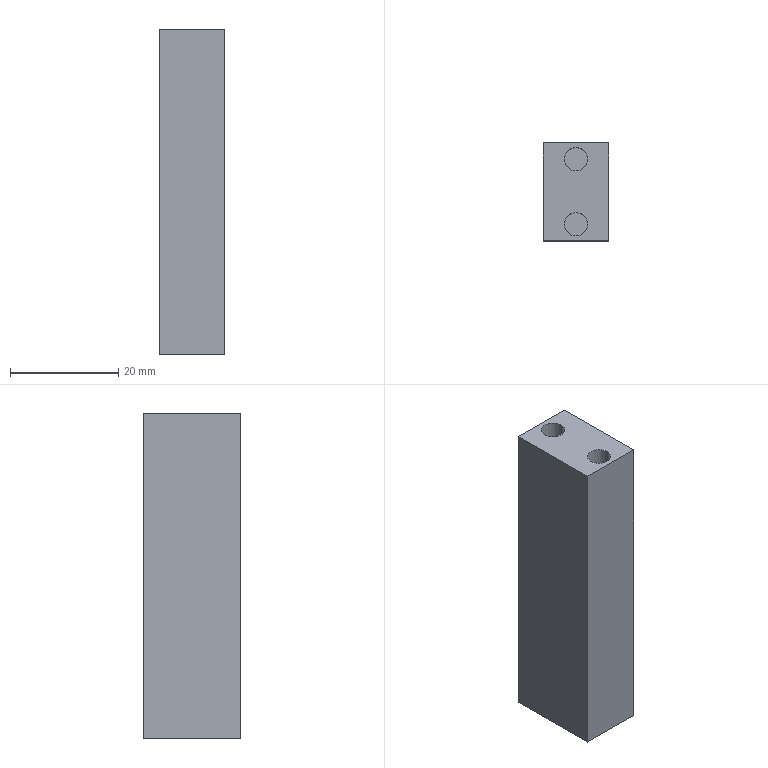Part | SolidWorks | features BaseBody 1 | 1 solid | 12 faces | box 12 x 18 x 60 mm | volume 12664 mm3 | plane 8 | cylinder 4 | commonest cylinder face diameters 4.3 x4
STEP:
#1=CARTESIAN_POINT('',(-2.15,6.,19.8));
#2=VERTEX_POINT('',#1);
#3=CARTESIAN_POINT('',(2.15,6.,19.8));
#4=VERTEX_POINT('',#3);
#5=CARTESIAN_POINT('',(0.,6.,19.8));
#6=DIRECTION('',(0.,0.,1.));
#7=DIRECTION('',(1.,0.,0.));
#8=AXIS2_PLACEMENT_3D('',#5,#6,#7);
#9=CIRCLE('',#8,2.15);
#10=EDGE_CURVE('',#2,#4,#9,.T.);
#11=ORIENTED_EDGE('',*,*,#10,.F.);
#12=CARTESIAN_POINT('',(-2.15,6.,30.));
#13=VERTEX_POINT('',#12);
#14=CARTESIAN_POINT('',(-2.15,6.,19.8));
#15=DIRECTION('',(0.,0.,1.));
#16=VECTOR('',#15,1000.);
#17=LINE('',#14,#16);
#18=EDGE_CURVE('',#2,#13,#17,.T.);
#19=ORIENTED_EDGE('',*,*,#18,.T.);
#20=CARTESIAN_POINT('',(2.15,6.,30.));
#21=VERTEX_POINT('',#20);
#22=CARTESIAN_POINT('',(0.,6.,30.));
#23=DIRECTION('',(0.,0.,-1.));
#24=DIRECTION('',(1.,0.,0.));
#25=AXIS2_PLACEMENT_3D('',#22,#23,#24);
#26=CIRCLE('',#25,2.15);
#27=EDGE_CURVE('',#21,#13,#26,.T.);
#28=ORIENTED_EDGE('',*,*,#27,.F.);
#29=CARTESIAN_POINT('',(2.15,6.,19.8));
#30=DIRECTION('',(0.,0.,1.));
#31=VECTOR('',#30,1000.);
#32=LINE('',#29,#31);
#33=EDGE_CURVE('',#4,#21,#32,.T.);
#34=ORIENTED_EDGE('',*,*,#33,.F.);
#35=EDGE_LOOP('',(#11,#19,#28,#34));
#36=FACE_OUTER_BOUND('',#35,.T.);
#37=CARTESIAN_POINT('',(0.,6.,19.8));
#38=DIRECTION('',(0.,0.,1.));
#39=DIRECTION('',(1.,0.,0.));
#40=AXIS2_PLACEMENT_3D('',#37,#38,#39);
#41=CYLINDRICAL_SURFACE('',#40,2.15);
#42=ADVANCED_FACE('',(#36),#41,.F.);
#43=CARTESIAN_POINT('',(-2.15,-6.,19.8));
#44=VERTEX_POINT('',#43);
#45=CARTESIAN_POINT('',(2.15,-6.,19.8));
#46=VERTEX_POINT('',#45);
#47=CARTESIAN_POINT('',(0.,-6.,19.8));
#48=DIRECTION('',(0.,0.,1.));
#49=DIRECTION('',(1.,0.,0.));
#50=AXIS2_PLACEMENT_3D('',#47,#48,#49);
#51=CIRCLE('',#50,2.15);
#52=EDGE_CURVE('',#44,#46,#51,.T.);
#53=ORIENTED_EDGE('',*,*,#52,.F.);
#54=CARTESIAN_POINT('',(-2.15,-6.,30.));
#55=VERTEX_POINT('',#54);
#56=CARTESIAN_POINT('',(-2.15,-6.,19.8));
#57=DIRECTION('',(0.,0.,1.));
#58=VECTOR('',#57,1000.);
#59=LINE('',#56,#58);
#60=EDGE_CURVE('',#44,#55,#59,.T.);
#61=ORIENTED_EDGE('',*,*,#60,.T.);
#62=CARTESIAN_POINT('',(2.15,-6.,30.));
#63=VERTEX_POINT('',#62);
#64=CARTESIAN_POINT('',(0.,-6.,30.));
#65=DIRECTION('',(0.,0.,-1.));
#66=DIRECTION('',(1.,0.,0.));
#67=AXIS2_PLACEMENT_3D('',#64,#65,#66);
#68=CIRCLE('',#67,2.15);
#69=EDGE_CURVE('',#63,#55,#68,.T.);
#70=ORIENTED_EDGE('',*,*,#69,.F.);
#71=CARTESIAN_POINT('',(2.15,-6.,19.8));
#72=DIRECTION('',(0.,0.,1.));
#73=VECTOR('',#72,1000.);
#74=LINE('',#71,#73);
#75=EDGE_CURVE('',#46,#63,#74,.T.);
#76=ORIENTED_EDGE('',*,*,#75,.F.);
#77=EDGE_LOOP('',(#53,#61,#70,#76));
#78=FACE_OUTER_BOUND('',#77,.T.);
#79=CARTESIAN_POINT('',(0.,-6.,19.8));
#80=DIRECTION('',(0.,0.,1.));
#81=DIRECTION('',(1.,0.,0.));
#82=AXIS2_PLACEMENT_3D('',#79,#80,#81);
#83=CYLINDRICAL_SURFACE('',#82,2.15);
#84=ADVANCED_FACE('',(#78),#83,.F.);
#85=CARTESIAN_POINT('',(-6.,9.,-30.));
#86=VERTEX_POINT('',#85);
#87=CARTESIAN_POINT('',(-6.,9.,30.));
#88=VERTEX_POINT('',#87);
#89=CARTESIAN_POINT('',(-6.,9.,-30.));
#90=DIRECTION('',(0.,0.,1.));
#91=VECTOR('',#90,1000.);
#92=LINE('',#89,#91);
#93=EDGE_CURVE('',#86,#88,#92,.T.);
#94=ORIENTED_EDGE('',*,*,#93,.F.);
#95=CARTESIAN_POINT('',(-6.,-9.,-30.));
#96=VERTEX_POINT('',#95);
#97=CARTESIAN_POINT('',(-6.,-9.,-30.));
#98=DIRECTION('',(0.,1.,0.));
#99=VECTOR('',#98,1000.);
#100=LINE('',#97,#99);
#101=EDGE_CURVE('',#96,#86,#100,.T.);
#102=ORIENTED_EDGE('',*,*,#101,.F.);
#103=CARTESIAN_POINT('',(-6.,-9.,30.));
#104=VERTEX_POINT('',#103);
#105=CARTESIAN_POINT('',(-6.,-9.,-30.));
#106=DIRECTION('',(0.,0.,-1.));
#107=VECTOR('',#106,1000.);
#108=LINE('',#105,#107);
#109=EDGE_CURVE('',#104,#96,#108,.T.);
#110=ORIENTED_EDGE('',*,*,#109,.F.);
#111=CARTESIAN_POINT('',(-6.,-9.,30.));
#112=DIRECTION('',(0.,-1.,0.));
#113=VECTOR('',#112,1000.);
#114=LINE('',#111,#113);
#115=EDGE_CURVE('',#88,#104,#114,.T.);
#116=ORIENTED_EDGE('',*,*,#115,.F.);
#117=EDGE_LOOP('',(#94,#102,#110,#116));
#118=FACE_OUTER_BOUND('',#117,.T.);
#119=CARTESIAN_POINT('',(-6.,-9.,-30.));
#120=DIRECTION('',(1.,0.,0.));
#121=DIRECTION('',(0.,0.,-1.));
#122=AXIS2_PLACEMENT_3D('',#119,#120,#121);
#123=PLANE('',#122);
#124=ADVANCED_FACE('',(#118),#123,.F.);
#125=ORIENTED_EDGE('',*,*,#27,.T.);
#126=CARTESIAN_POINT('',(0.,6.,30.));
#127=DIRECTION('',(0.,0.,-1.));
#128=DIRECTION('',(1.,0.,0.));
#129=AXIS2_PLACEMENT_3D('',#126,#127,#128);
#130=CIRCLE('',#129,2.15);
#131=EDGE_CURVE('',#13,#21,#130,.T.);
#132=ORIENTED_EDGE('',*,*,#131,.T.);
#133=EDGE_LOOP('',(#125,#132));
#134=FACE_BOUND('',#133,.T.);
#135=ORIENTED_EDGE('',*,*,#69,.T.);
#136=CARTESIAN_POINT('',(0.,-6.,30.));
#137=DIRECTION('',(0.,0.,-1.));
#138=DIRECTION('',(1.,0.,0.));
#139=AXIS2_PLACEMENT_3D('',#136,#137,#138);
#140=CIRCLE('',#139,2.15);
#141=EDGE_CURVE('',#55,#63,#140,.T.);
#142=ORIENTED_EDGE('',*,*,#141,.T.);
#143=EDGE_LOOP('',(#135,#142));
#144=FACE_BOUND('',#143,.T.);
#145=CARTESIAN_POINT('',(6.,-9.,30.));
#146=VERTEX_POINT('',#145);
#147=CARTESIAN_POINT('',(6.,9.,30.));
#148=VERTEX_POINT('',#147);
#149=CARTESIAN_POINT('',(6.,-9.,30.));
#150=DIRECTION('',(0.,1.,0.));
#151=VECTOR('',#150,1000.);
#152=LINE('',#149,#151);
#153=EDGE_CURVE('',#146,#148,#152,.T.);
#154=ORIENTED_EDGE('',*,*,#153,.T.);
#155=CARTESIAN_POINT('',(-6.,9.,30.));
#156=DIRECTION('',(-1.,0.,0.));
#157=VECTOR('',#156,1000.);
#158=LINE('',#155,#157);
#159=EDGE_CURVE('',#148,#88,#158,.T.);
#160=ORIENTED_EDGE('',*,*,#159,.T.);
#161=ORIENTED_EDGE('',*,*,#115,.T.);
#162=CARTESIAN_POINT('',(-6.,-9.,30.));
#163=DIRECTION('',(1.,0.,0.));
#164=VECTOR('',#163,1000.);
#165=LINE('',#162,#164);
#166=EDGE_CURVE('',#104,#146,#165,.T.);
#167=ORIENTED_EDGE('',*,*,#166,.T.);
#168=EDGE_LOOP('',(#154,#160,#161,#167));
#169=FACE_OUTER_BOUND('',#168,.T.);
#170=CARTESIAN_POINT('',(-6.,-9.,30.));
#171=DIRECTION('',(0.,0.,1.));
#172=DIRECTION('',(1.,0.,0.));
#173=AXIS2_PLACEMENT_3D('',#170,#171,#172);
#174=PLANE('',#173);
#175=ADVANCED_FACE('',(#134,#144,#169),#174,.T.);
#176=ORIENTED_EDGE('',*,*,#159,.F.);
#177=CARTESIAN_POINT('',(6.,9.,-30.));
#178=VERTEX_POINT('',#177);
#179=CARTESIAN_POINT('',(6.,9.,-30.));
#180=DIRECTION('',(0.,0.,-1.));
#181=VECTOR('',#180,1000.);
#182=LINE('',#179,#181);
#183=EDGE_CURVE('',#148,#178,#182,.T.);
#184=ORIENTED_EDGE('',*,*,#183,.T.);
#185=CARTESIAN_POINT('',(-6.,9.,-30.));
#186=DIRECTION('',(-1.,0.,0.));
#187=VECTOR('',#186,1000.);
#188=LINE('',#185,#187);
#189=EDGE_CURVE('',#178,#86,#188,.T.);
#190=ORIENTED_EDGE('',*,*,#189,.T.);
#191=ORIENTED_EDGE('',*,*,#93,.T.);
#192=EDGE_LOOP('',(#176,#184,#190,#191));
#193=FACE_OUTER_BOUND('',#192,.T.);
#194=CARTESIAN_POINT('',(-6.,9.,-30.));
#195=DIRECTION('',(0.,1.,0.));
#196=DIRECTION('',(0.,0.,1.));
#197=AXIS2_PLACEMENT_3D('',#194,#195,#196);
#198=PLANE('',#197);
#199=ADVANCED_FACE('',(#193),#198,.T.);
#200=CARTESIAN_POINT('',(6.,-9.,-30.));
#201=VERTEX_POINT('',#200);
#202=CARTESIAN_POINT('',(6.,-9.,-30.));
#203=DIRECTION('',(0.,1.,0.));
#204=VECTOR('',#203,1000.);
#205=LINE('',#202,#204);
#206=EDGE_CURVE('',#201,#178,#205,.T.);
#207=ORIENTED_EDGE('',*,*,#206,.F.);
#208=CARTESIAN_POINT('',(-6.,-9.,-30.));
#209=DIRECTION('',(1.,0.,0.));
#210=VECTOR('',#209,1000.);
#211=LINE('',#208,#210);
#212=EDGE_CURVE('',#96,#201,#211,.T.);
#213=ORIENTED_EDGE('',*,*,#212,.F.);
#214=ORIENTED_EDGE('',*,*,#101,.T.);
#215=ORIENTED_EDGE('',*,*,#189,.F.);
#216=EDGE_LOOP('',(#207,#213,#214,#215));
#217=FACE_OUTER_BOUND('',#216,.T.);
#218=CARTESIAN_POINT('',(-6.,-9.,-30.));
#219=DIRECTION('',(0.,0.,1.));
#220=DIRECTION('',(1.,0.,0.));
#221=AXIS2_PLACEMENT_3D('',#218,#219,#220);
#222=PLANE('',#221);
#223=ADVANCED_FACE('',(#217),#222,.F.);
#224=ORIENTED_EDGE('',*,*,#166,.F.);
#225=ORIENTED_EDGE('',*,*,#109,.T.);
#226=ORIENTED_EDGE('',*,*,#212,.T.);
#227=CARTESIAN_POINT('',(6.,-9.,-30.));
#228=DIRECTION('',(0.,0.,-1.));
#229=VECTOR('',#228,1000.);
#230=LINE('',#227,#229);
#231=EDGE_CURVE('',#146,#201,#230,.T.);
#232=ORIENTED_EDGE('',*,*,#231,.F.);
#233=EDGE_LOOP('',(#224,#225,#226,#232));
#234=FACE_OUTER_BOUND('',#233,.T.);
#235=CARTESIAN_POINT('',(-6.,-9.,-30.));
#236=DIRECTION('',(0.,1.,0.));
#237=DIRECTION('',(0.,0.,1.));
#238=AXIS2_PLACEMENT_3D('',#235,#236,#237);
#239=PLANE('',#238);
#240=ADVANCED_FACE('',(#234),#239,.F.);
#241=ORIENTED_EDGE('',*,*,#18,.F.);
#242=CARTESIAN_POINT('',(0.,6.,19.8));
#243=DIRECTION('',(0.,0.,1.));
#244=DIRECTION('',(1.,0.,0.));
#245=AXIS2_PLACEMENT_3D('',#242,#243,#244);
#246=CIRCLE('',#245,2.15);
#247=EDGE_CURVE('',#4,#2,#246,.T.);
#248=ORIENTED_EDGE('',*,*,#247,.F.);
#249=ORIENTED_EDGE('',*,*,#33,.T.);
#250=ORIENTED_EDGE('',*,*,#131,.F.);
#251=EDGE_LOOP('',(#241,#248,#249,#250));
#252=FACE_OUTER_BOUND('',#251,.T.);
#253=CARTESIAN_POINT('',(0.,6.,19.8));
#254=DIRECTION('',(0.,0.,1.));
#255=DIRECTION('',(1.,0.,0.));
#256=AXIS2_PLACEMENT_3D('',#253,#254,#255);
#257=CYLINDRICAL_SURFACE('',#256,2.15);
#258=ADVANCED_FACE('',(#252),#257,.F.);
#259=ORIENTED_EDGE('',*,*,#60,.F.);
#260=CARTESIAN_POINT('',(0.,-6.,19.8));
#261=DIRECTION('',(0.,0.,1.));
#262=DIRECTION('',(1.,0.,0.));
#263=AXIS2_PLACEMENT_3D('',#260,#261,#262);
#264=CIRCLE('',#263,2.15);
#265=EDGE_CURVE('',#46,#44,#264,.T.);
#266=ORIENTED_EDGE('',*,*,#265,.F.);
#267=ORIENTED_EDGE('',*,*,#75,.T.);
#268=ORIENTED_EDGE('',*,*,#141,.F.);
#269=EDGE_LOOP('',(#259,#266,#267,#268));
#270=FACE_OUTER_BOUND('',#269,.T.);
#271=CARTESIAN_POINT('',(0.,-6.,19.8));
#272=DIRECTION('',(0.,0.,1.));
#273=DIRECTION('',(1.,0.,0.));
#274=AXIS2_PLACEMENT_3D('',#271,#272,#273);
#275=CYLINDRICAL_SURFACE('',#274,2.15);
#276=ADVANCED_FACE('',(#270),#275,.F.);
#277=ORIENTED_EDGE('',*,*,#183,.F.);
#278=ORIENTED_EDGE('',*,*,#153,.F.);
#279=ORIENTED_EDGE('',*,*,#231,.T.);
#280=ORIENTED_EDGE('',*,*,#206,.T.);
#281=EDGE_LOOP('',(#277,#278,#279,#280));
#282=FACE_OUTER_BOUND('',#281,.T.);
#283=CARTESIAN_POINT('',(6.,-9.,-30.));
#284=DIRECTION('',(1.,0.,0.));
#285=DIRECTION('',(0.,0.,-1.));
#286=AXIS2_PLACEMENT_3D('',#283,#284,#285);
#287=PLANE('',#286);
#288=ADVANCED_FACE('',(#282),#287,.T.);
#289=ORIENTED_EDGE('',*,*,#247,.T.);
#290=ORIENTED_EDGE('',*,*,#10,.T.);
#291=EDGE_LOOP('',(#289,#290));
#292=FACE_OUTER_BOUND('',#291,.T.);
#293=CARTESIAN_POINT('',(0.,6.,19.8));
#294=DIRECTION('',(0.,0.,1.));
#295=DIRECTION('',(1.,0.,0.));
#296=AXIS2_PLACEMENT_3D('',#293,#294,#295);
#297=PLANE('',#296);
#298=ADVANCED_FACE('',(#292),#297,.T.);
#299=ORIENTED_EDGE('',*,*,#265,.T.);
#300=ORIENTED_EDGE('',*,*,#52,.T.);
#301=EDGE_LOOP('',(#299,#300));
#302=FACE_OUTER_BOUND('',#301,.T.);
#303=CARTESIAN_POINT('',(0.,-6.,19.8));
#304=DIRECTION('',(0.,0.,1.));
#305=DIRECTION('',(1.,0.,0.));
#306=AXIS2_PLACEMENT_3D('',#303,#304,#305);
#307=PLANE('',#306);
#308=ADVANCED_FACE('',(#302),#307,.T.);
#309=CLOSED_SHELL('',(#42,#84,#124,#175,#199,#223,#240,#258,#276,#288,#298,#308));
#310=MANIFOLD_SOLID_BREP('',#309);
#311=CARTESIAN_POINT('',(0.,0.,0.));
#312=DIRECTION('',(0.,0.,1.));
#313=DIRECTION('',(1.,0.,0.));
#314=AXIS2_PLACEMENT_3D('',#311,#312,#313);
#315=(LENGTH_UNIT()NAMED_UNIT(*)SI_UNIT(.MILLI.,.METRE.));
#316=UNCERTAINTY_MEASURE_WITH_UNIT(LENGTH_MEASURE(0.00001),#315,'','');
#317=(NAMED_UNIT(*)PLANE_ANGLE_UNIT()SI_UNIT($,.RADIAN.));
#318=(NAMED_UNIT(*)SI_UNIT($,.STERADIAN.)SOLID_ANGLE_UNIT());
#319=(GEOMETRIC_REPRESENTATION_CONTEXT(3)GLOBAL_UNCERTAINTY_ASSIGNED_CONTEXT((#316))GLOBAL_UNIT_ASSIGNED_CONTEXT((#315,#317,#318))REPRESENTATION_CONTEXT('',''));
#320=ADVANCED_BREP_SHAPE_REPRESENTATION('',(#310,#314),#319);